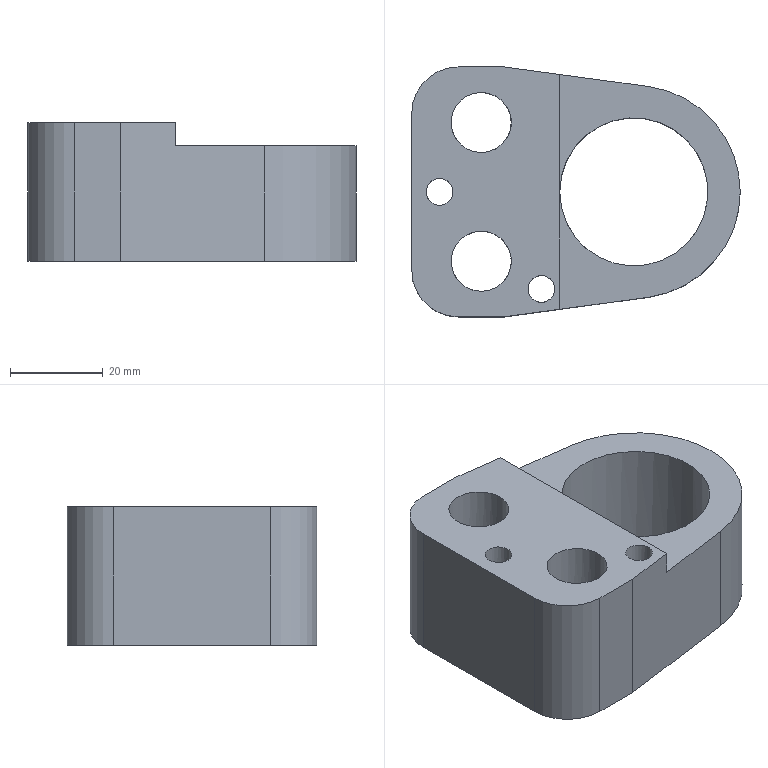Part | NX | features solid 2 | 1 solid | 25 faces | box 71.007 x 54.004 x 30 mm | volume 55355 mm3 | plane 13 | cylinder 12 | commonest cylinder face diameters 5.8 x2 8 x2 13 x2 19 x2 20 x2 32 x1
STEP:
#1=CARTESIAN_POINT('',(-440.164,-179.961,113.));
#2=VERTEX_POINT('',#1);
#3=CARTESIAN_POINT('',(-428.165,-178.332,113.));
#4=VERTEX_POINT('',#3);
#5=CARTESIAN_POINT('',(-420.346,-177.27,113.));
#6=DIRECTION('',(0.9909,0.1345,0.));
#7=VECTOR('',#6,1000.);
#8=LINE('',#5,#7);
#9=EDGE_CURVE('',#2,#4,#8,.T.);
#10=ORIENTED_EDGE('',*,*,#9,.T.);
#11=CARTESIAN_POINT('',(-428.185,-127.581,113.));
#12=VERTEX_POINT('',#11);
#13=CARTESIAN_POINT('',(-428.175,-152.956,113.));
#14=DIRECTION('',(-0.000407,1.,0.));
#15=VECTOR('',#14,1000.);
#16=LINE('',#13,#15);
#17=EDGE_CURVE('',#4,#12,#16,.T.);
#18=ORIENTED_EDGE('',*,*,#17,.T.);
#19=CARTESIAN_POINT('',(-440.186,-125.961,113.));
#20=VERTEX_POINT('',#19);
#21=CARTESIAN_POINT('',(-420.366,-128.636,113.));
#22=DIRECTION('',(-0.991,0.1337,0.));
#23=VECTOR('',#22,1000.);
#24=LINE('',#21,#23);
#25=EDGE_CURVE('',#12,#20,#24,.T.);
#26=ORIENTED_EDGE('',*,*,#25,.T.);
#27=CARTESIAN_POINT('',(-450.186,-125.965,113.));
#28=VERTEX_POINT('',#27);
#29=CARTESIAN_POINT('',(-424.641,-125.955,113.));
#30=DIRECTION('',(1.,0.000407,0.));
#31=VECTOR('',#30,1000.);
#32=LINE('',#29,#31);
#33=EDGE_CURVE('',#28,#20,#32,.T.);
#34=ORIENTED_EDGE('',*,*,#33,.F.);
#35=CARTESIAN_POINT('',(-460.182,-135.969,113.));
#36=VERTEX_POINT('',#35);
#37=CARTESIAN_POINT('',(-450.182,-135.965,113.));
#38=DIRECTION('',(0.,0.,1.));
#39=DIRECTION('',(1.,0.,0.));
#40=AXIS2_PLACEMENT_3D('',#37,#38,#39);
#41=CIRCLE('',#40,10.);
#42=EDGE_CURVE('',#28,#36,#41,.T.);
#43=ORIENTED_EDGE('',*,*,#42,.T.);
#44=CARTESIAN_POINT('',(-460.168,-169.969,113.));
#45=VERTEX_POINT('',#44);
#46=CARTESIAN_POINT('',(-460.175,-152.969,113.));
#47=DIRECTION('',(-0.000407,1.,0.));
#48=VECTOR('',#47,1000.);
#49=LINE('',#46,#48);
#50=EDGE_CURVE('',#45,#36,#49,.T.);
#51=ORIENTED_EDGE('',*,*,#50,.F.);
#52=CARTESIAN_POINT('',(-450.164,-179.965,113.));
#53=VERTEX_POINT('',#52);
#54=CARTESIAN_POINT('',(-450.168,-169.965,113.));
#55=DIRECTION('',(0.,0.,1.));
#56=DIRECTION('',(1.,0.,0.));
#57=AXIS2_PLACEMENT_3D('',#54,#55,#56);
#58=CIRCLE('',#57,10.);
#59=EDGE_CURVE('',#45,#53,#58,.T.);
#60=ORIENTED_EDGE('',*,*,#59,.T.);
#61=CARTESIAN_POINT('',(-424.619,-179.955,113.));
#62=DIRECTION('',(-1.,-0.000407,0.));
#63=VECTOR('',#62,1000.);
#64=LINE('',#61,#63);
#65=EDGE_CURVE('',#2,#53,#64,.T.);
#66=ORIENTED_EDGE('',*,*,#65,.F.);
#67=EDGE_LOOP('',(#10,#18,#26,#34,#43,#51,#60,#66));
#68=FACE_BOUND('',#67,.T.);
#69=CARTESIAN_POINT('',(-454.176,-150.067,113.));
#70=VERTEX_POINT('',#69);
#71=CARTESIAN_POINT('',(-454.175,-152.967,113.));
#72=DIRECTION('',(0.,0.,-1.));
#73=DIRECTION('',(-0.000407,1.,0.));
#74=AXIS2_PLACEMENT_3D('',#71,#72,#73);
#75=CIRCLE('',#74,2.9);
#76=EDGE_CURVE('',#70,#70,#75,.T.);
#77=ORIENTED_EDGE('',*,*,#76,.T.);
#78=EDGE_LOOP('',(#77));
#79=FACE_BOUND('',#78,.T.);
#80=CARTESIAN_POINT('',(-432.168,-171.058,113.));
#81=VERTEX_POINT('',#80);
#82=CARTESIAN_POINT('',(-432.167,-173.958,113.));
#83=DIRECTION('',(0.,0.,-1.));
#84=DIRECTION('',(-0.000407,1.,0.));
#85=AXIS2_PLACEMENT_3D('',#82,#83,#84);
#86=CIRCLE('',#85,2.9);
#87=EDGE_CURVE('',#81,#81,#86,.T.);
#88=ORIENTED_EDGE('',*,*,#87,.T.);
#89=EDGE_LOOP('',(#88));
#90=FACE_BOUND('',#89,.T.);
#91=CARTESIAN_POINT('',(-445.172,-161.463,113.));
#92=VERTEX_POINT('',#91);
#93=CARTESIAN_POINT('',(-445.169,-167.963,113.));
#94=DIRECTION('',(0.,0.,-1.));
#95=DIRECTION('',(-0.000407,1.,0.));
#96=AXIS2_PLACEMENT_3D('',#93,#94,#95);
#97=CIRCLE('',#96,6.5);
#98=EDGE_CURVE('',#92,#92,#97,.T.);
#99=ORIENTED_EDGE('',*,*,#98,.T.);
#100=EDGE_LOOP('',(#99));
#101=FACE_BOUND('',#100,.T.);
#102=CARTESIAN_POINT('',(-445.184,-131.463,113.));
#103=VERTEX_POINT('',#102);
#104=CARTESIAN_POINT('',(-445.181,-137.963,113.));
#105=DIRECTION('',(0.,0.,-1.));
#106=DIRECTION('',(-0.000407,1.,0.));
#107=AXIS2_PLACEMENT_3D('',#104,#105,#106);
#108=CIRCLE('',#107,6.5);
#109=EDGE_CURVE('',#103,#103,#108,.T.);
#110=ORIENTED_EDGE('',*,*,#109,.T.);
#111=EDGE_LOOP('',(#110));
#112=FACE_BOUND('',#111,.T.);
#113=CARTESIAN_POINT('',(-424.63,-152.955,113.));
#114=DIRECTION('',(0.,0.,1.));
#115=DIRECTION('',(0.000407,-1.,0.));
#116=AXIS2_PLACEMENT_3D('',#113,#114,#115);
#117=PLANE('',#116);
#118=ADVANCED_FACE('',(#68,#79,#90,#101,#112),#117,.T.);
#119=CARTESIAN_POINT('',(-440.186,-125.961,83.));
#120=VERTEX_POINT('',#119);
#121=CARTESIAN_POINT('',(-440.186,-125.961,83.));
#122=DIRECTION('',(0.,0.,1.));
#123=VECTOR('',#122,1000.);
#124=LINE('',#121,#123);
#125=EDGE_CURVE('',#120,#20,#124,.T.);
#126=ORIENTED_EDGE('',*,*,#125,.F.);
#127=CARTESIAN_POINT('',(-450.186,-125.965,83.));
#128=VERTEX_POINT('',#127);
#129=CARTESIAN_POINT('',(-424.641,-125.955,83.));
#130=DIRECTION('',(-1.,-0.000407,0.));
#131=VECTOR('',#130,1000.);
#132=LINE('',#129,#131);
#133=EDGE_CURVE('',#120,#128,#132,.T.);
#134=ORIENTED_EDGE('',*,*,#133,.T.);
#135=CARTESIAN_POINT('',(-450.186,-125.965,83.));
#136=DIRECTION('',(0.,0.,1.));
#137=VECTOR('',#136,1000.);
#138=LINE('',#135,#137);
#139=EDGE_CURVE('',#128,#28,#138,.T.);
#140=ORIENTED_EDGE('',*,*,#139,.T.);
#141=ORIENTED_EDGE('',*,*,#33,.T.);
#142=EDGE_LOOP('',(#126,#134,#140,#141));
#143=FACE_BOUND('',#142,.T.);
#144=CARTESIAN_POINT('',(-424.641,-125.955,83.));
#145=DIRECTION('',(-0.000407,1.,0.));
#146=DIRECTION('',(0.,0.,1.));
#147=AXIS2_PLACEMENT_3D('',#144,#145,#146);
#148=PLANE('',#147);
#149=ADVANCED_FACE('',(#143),#148,.T.);
#150=CARTESIAN_POINT('',(-409.076,-175.74,83.));
#151=VERTEX_POINT('',#150);
#152=CARTESIAN_POINT('',(-440.164,-179.961,83.));
#153=VERTEX_POINT('',#152);
#154=CARTESIAN_POINT('',(-420.346,-177.27,83.));
#155=DIRECTION('',(-0.9909,-0.1345,0.));
#156=VECTOR('',#155,1000.);
#157=LINE('',#154,#156);
#158=EDGE_CURVE('',#151,#153,#157,.T.);
#159=ORIENTED_EDGE('',*,*,#158,.T.);
#160=CARTESIAN_POINT('',(-450.164,-179.965,83.));
#161=VERTEX_POINT('',#160);
#162=CARTESIAN_POINT('',(-424.619,-179.955,83.));
#163=DIRECTION('',(1.,0.000407,0.));
#164=VECTOR('',#163,1000.);
#165=LINE('',#162,#164);
#166=EDGE_CURVE('',#161,#153,#165,.T.);
#167=ORIENTED_EDGE('',*,*,#166,.F.);
#168=CARTESIAN_POINT('',(-460.168,-169.969,83.));
#169=VERTEX_POINT('',#168);
#170=CARTESIAN_POINT('',(-450.168,-169.965,83.));
#171=DIRECTION('',(0.,0.,-1.));
#172=DIRECTION('',(-1.,0.,0.));
#173=AXIS2_PLACEMENT_3D('',#170,#171,#172);
#174=CIRCLE('',#173,10.);
#175=EDGE_CURVE('',#161,#169,#174,.T.);
#176=ORIENTED_EDGE('',*,*,#175,.T.);
#177=CARTESIAN_POINT('',(-460.182,-135.969,83.));
#178=VERTEX_POINT('',#177);
#179=CARTESIAN_POINT('',(-460.175,-152.969,83.));
#180=DIRECTION('',(0.000407,-1.,0.));
#181=VECTOR('',#180,1000.);
#182=LINE('',#179,#181);
#183=EDGE_CURVE('',#178,#169,#182,.T.);
#184=ORIENTED_EDGE('',*,*,#183,.F.);
#185=CARTESIAN_POINT('',(-450.182,-135.965,83.));
#186=DIRECTION('',(0.,0.,-1.));
#187=DIRECTION('',(-1.,0.,0.));
#188=AXIS2_PLACEMENT_3D('',#185,#186,#187);
#189=CIRCLE('',#188,10.);
#190=EDGE_CURVE('',#178,#128,#189,.T.);
#191=ORIENTED_EDGE('',*,*,#190,.T.);
#192=ORIENTED_EDGE('',*,*,#133,.F.);
#193=CARTESIAN_POINT('',(-409.094,-130.157,83.));
#194=VERTEX_POINT('',#193);
#195=CARTESIAN_POINT('',(-420.366,-128.636,83.));
#196=DIRECTION('',(0.991,-0.1337,0.));
#197=VECTOR('',#196,1000.);
#198=LINE('',#195,#197);
#199=EDGE_CURVE('',#120,#194,#198,.T.);
#200=ORIENTED_EDGE('',*,*,#199,.T.);
#201=CARTESIAN_POINT('',(-412.175,-152.95,83.));
#202=DIRECTION('',(0.,0.,1.));
#203=DIRECTION('',(0.000407,-1.,0.));
#204=AXIS2_PLACEMENT_3D('',#201,#202,#203);
#205=CIRCLE('',#204,23.);
#206=EDGE_CURVE('',#151,#194,#205,.T.);
#207=ORIENTED_EDGE('',*,*,#206,.F.);
#208=EDGE_LOOP('',(#159,#167,#176,#184,#191,#192,#200,#207));
#209=FACE_BOUND('',#208,.T.);
#210=CARTESIAN_POINT('',(-454.174,-156.967,83.));
#211=VERTEX_POINT('',#210);
#212=CARTESIAN_POINT('',(-454.175,-152.967,83.));
#213=DIRECTION('',(0.,0.,1.));
#214=DIRECTION('',(0.000407,-1.,0.));
#215=AXIS2_PLACEMENT_3D('',#212,#213,#214);
#216=CIRCLE('',#215,4.);
#217=EDGE_CURVE('',#211,#211,#216,.T.);
#218=ORIENTED_EDGE('',*,*,#217,.T.);
#219=EDGE_LOOP('',(#218));
#220=FACE_BOUND('',#219,.T.);
#221=CARTESIAN_POINT('',(-432.165,-177.958,83.));
#222=VERTEX_POINT('',#221);
#223=CARTESIAN_POINT('',(-432.167,-173.958,83.));
#224=DIRECTION('',(0.,0.,1.));
#225=DIRECTION('',(0.000407,-1.,0.));
#226=AXIS2_PLACEMENT_3D('',#223,#224,#225);
#227=CIRCLE('',#226,4.);
#228=EDGE_CURVE('',#222,#222,#227,.T.);
#229=ORIENTED_EDGE('',*,*,#228,.T.);
#230=EDGE_LOOP('',(#229));
#231=FACE_BOUND('',#230,.T.);
#232=CARTESIAN_POINT('',(-445.165,-177.463,83.));
#233=VERTEX_POINT('',#232);
#234=CARTESIAN_POINT('',(-445.169,-167.963,83.));
#235=DIRECTION('',(0.,0.,1.));
#236=DIRECTION('',(0.000407,-1.,0.));
#237=AXIS2_PLACEMENT_3D('',#234,#235,#236);
#238=CIRCLE('',#237,9.5);
#239=EDGE_CURVE('',#233,#233,#238,.T.);
#240=ORIENTED_EDGE('',*,*,#239,.T.);
#241=EDGE_LOOP('',(#240));
#242=FACE_BOUND('',#241,.T.);
#243=CARTESIAN_POINT('',(-445.177,-147.463,83.));
#244=VERTEX_POINT('',#243);
#245=CARTESIAN_POINT('',(-445.181,-137.963,83.));
#246=DIRECTION('',(0.,0.,1.));
#247=DIRECTION('',(0.000407,-1.,0.));
#248=AXIS2_PLACEMENT_3D('',#245,#246,#247);
#249=CIRCLE('',#248,9.5);
#250=EDGE_CURVE('',#244,#244,#249,.T.);
#251=ORIENTED_EDGE('',*,*,#250,.T.);
#252=EDGE_LOOP('',(#251));
#253=FACE_BOUND('',#252,.T.);
#254=CARTESIAN_POINT('',(-412.169,-168.95,83.));
#255=VERTEX_POINT('',#254);
#256=CARTESIAN_POINT('',(-412.175,-152.95,83.));
#257=DIRECTION('',(0.,0.,1.));
#258=DIRECTION('',(0.000407,-1.,0.));
#259=AXIS2_PLACEMENT_3D('',#256,#257,#258);
#260=CIRCLE('',#259,16.);
#261=EDGE_CURVE('',#255,#255,#260,.T.);
#262=ORIENTED_EDGE('',*,*,#261,.T.);
#263=EDGE_LOOP('',(#262));
#264=FACE_BOUND('',#263,.T.);
#265=CARTESIAN_POINT('',(-424.63,-152.955,83.));
#266=DIRECTION('',(0.,0.,-1.));
#267=DIRECTION('',(-0.000407,1.,0.));
#268=AXIS2_PLACEMENT_3D('',#265,#266,#267);
#269=PLANE('',#268);
#270=ADVANCED_FACE('',(#209,#220,#231,#242,#253,#264),#269,.T.);
#271=CARTESIAN_POINT('',(-440.164,-179.961,83.));
#272=DIRECTION('',(0.,0.,1.));
#273=VECTOR('',#272,1000.);
#274=LINE('',#271,#273);
#275=EDGE_CURVE('',#153,#2,#274,.T.);
#276=ORIENTED_EDGE('',*,*,#275,.T.);
#277=ORIENTED_EDGE('',*,*,#65,.T.);
#278=CARTESIAN_POINT('',(-450.164,-179.965,83.));
#279=DIRECTION('',(0.,0.,1.));
#280=VECTOR('',#279,1000.);
#281=LINE('',#278,#280);
#282=EDGE_CURVE('',#53,#161,#281,.F.);
#283=ORIENTED_EDGE('',*,*,#282,.T.);
#284=ORIENTED_EDGE('',*,*,#166,.T.);
#285=EDGE_LOOP('',(#276,#277,#283,#284));
#286=FACE_BOUND('',#285,.T.);
#287=CARTESIAN_POINT('',(-424.619,-179.955,83.));
#288=DIRECTION('',(0.000407,-1.,0.));
#289=DIRECTION('',(0.,0.,-1.));
#290=AXIS2_PLACEMENT_3D('',#287,#288,#289);
#291=PLANE('',#290);
#292=ADVANCED_FACE('',(#286),#291,.T.);
#293=CARTESIAN_POINT('',(-409.076,-175.74,108.));
#294=VERTEX_POINT('',#293);
#295=CARTESIAN_POINT('',(-409.094,-130.157,108.));
#296=VERTEX_POINT('',#295);
#297=CARTESIAN_POINT('',(-412.175,-152.95,108.));
#298=DIRECTION('',(0.,0.,-1.));
#299=DIRECTION('',(-1.,0.,0.));
#300=AXIS2_PLACEMENT_3D('',#297,#298,#299);
#301=CIRCLE('',#300,23.);
#302=EDGE_CURVE('',#294,#296,#301,.F.);
#303=ORIENTED_EDGE('',*,*,#302,.F.);
#304=CARTESIAN_POINT('',(-409.076,-175.74,113.));
#305=DIRECTION('',(0.,0.,-1.));
#306=VECTOR('',#305,1000.);
#307=LINE('',#304,#306);
#308=EDGE_CURVE('',#294,#151,#307,.T.);
#309=ORIENTED_EDGE('',*,*,#308,.T.);
#310=ORIENTED_EDGE('',*,*,#206,.T.);
#311=CARTESIAN_POINT('',(-409.094,-130.157,113.));
#312=DIRECTION('',(0.,0.,-1.));
#313=VECTOR('',#312,1000.);
#314=LINE('',#311,#313);
#315=EDGE_CURVE('',#194,#296,#314,.F.);
#316=ORIENTED_EDGE('',*,*,#315,.T.);
#317=EDGE_LOOP('',(#303,#309,#310,#316));
#318=FACE_BOUND('',#317,.T.);
#319=CARTESIAN_POINT('',(-412.175,-152.95,113.));
#320=DIRECTION('',(0.,0.,-1.));
#321=DIRECTION('',(-0.000407,1.,0.));
#322=AXIS2_PLACEMENT_3D('',#319,#320,#321);
#323=CYLINDRICAL_SURFACE('',#322,23.);
#324=ADVANCED_FACE('',(#318),#323,.T.);
#325=ORIENTED_EDGE('',*,*,#183,.T.);
#326=CARTESIAN_POINT('',(-460.168,-169.969,83.));
#327=DIRECTION('',(0.,0.,1.));
#328=VECTOR('',#327,1000.);
#329=LINE('',#326,#328);
#330=EDGE_CURVE('',#169,#45,#329,.T.);
#331=ORIENTED_EDGE('',*,*,#330,.T.);
#332=ORIENTED_EDGE('',*,*,#50,.T.);
#333=CARTESIAN_POINT('',(-460.182,-135.969,83.));
#334=DIRECTION('',(0.,0.,1.));
#335=VECTOR('',#334,1000.);
#336=LINE('',#333,#335);
#337=EDGE_CURVE('',#36,#178,#336,.F.);
#338=ORIENTED_EDGE('',*,*,#337,.T.);
#339=EDGE_LOOP('',(#325,#331,#332,#338));
#340=FACE_BOUND('',#339,.T.);
#341=CARTESIAN_POINT('',(-460.175,-152.969,83.));
#342=DIRECTION('',(-1.,-0.000407,0.));
#343=DIRECTION('',(0.,0.,-1.));
#344=AXIS2_PLACEMENT_3D('',#341,#342,#343);
#345=PLANE('',#344);
#346=ADVANCED_FACE('',(#340),#345,.T.);
#347=ORIENTED_EDGE('',*,*,#17,.F.);
#348=CARTESIAN_POINT('',(-428.165,-178.332,108.));
#349=VERTEX_POINT('',#348);
#350=CARTESIAN_POINT('',(-428.165,-178.332,108.));
#351=DIRECTION('',(0.,0.,-1.));
#352=VECTOR('',#351,1000.);
#353=LINE('',#350,#352);
#354=EDGE_CURVE('',#4,#349,#353,.T.);
#355=ORIENTED_EDGE('',*,*,#354,.T.);
#356=CARTESIAN_POINT('',(-428.175,-152.956,108.));
#357=VERTEX_POINT('',#356);
#358=CARTESIAN_POINT('',(-428.175,-152.956,108.));
#359=DIRECTION('',(0.000407,-1.,0.));
#360=VECTOR('',#359,1000.);
#361=LINE('',#358,#360);
#362=EDGE_CURVE('',#357,#349,#361,.T.);
#363=ORIENTED_EDGE('',*,*,#362,.F.);
#364=CARTESIAN_POINT('',(-428.185,-127.581,108.));
#365=VERTEX_POINT('',#364);
#366=CARTESIAN_POINT('',(-428.175,-152.956,108.));
#367=DIRECTION('',(0.000407,-1.,0.));
#368=VECTOR('',#367,1000.);
#369=LINE('',#366,#368);
#370=EDGE_CURVE('',#365,#357,#369,.T.);
#371=ORIENTED_EDGE('',*,*,#370,.F.);
#372=CARTESIAN_POINT('',(-428.185,-127.581,108.));
#373=DIRECTION('',(0.,0.,1.));
#374=VECTOR('',#373,1000.);
#375=LINE('',#372,#374);
#376=EDGE_CURVE('',#365,#12,#375,.T.);
#377=ORIENTED_EDGE('',*,*,#376,.T.);
#378=EDGE_LOOP('',(#347,#355,#363,#371,#377));
#379=FACE_BOUND('',#378,.T.);
#380=CARTESIAN_POINT('',(-428.175,-152.956,108.));
#381=DIRECTION('',(-1.,-0.000407,0.));
#382=DIRECTION('',(0.,0.,-1.));
#383=AXIS2_PLACEMENT_3D('',#380,#381,#382);
#384=PLANE('',#383);
#385=ADVANCED_FACE('',(#379),#384,.F.);
#386=ORIENTED_EDGE('',*,*,#362,.T.);
#387=CARTESIAN_POINT('',(-397.788,-174.207,108.));
#388=DIRECTION('',(0.9909,0.1345,0.));
#389=VECTOR('',#388,1000.);
#390=LINE('',#387,#389);
#391=EDGE_CURVE('',#349,#294,#390,.T.);
#392=ORIENTED_EDGE('',*,*,#391,.T.);
#393=ORIENTED_EDGE('',*,*,#302,.T.);
#394=CARTESIAN_POINT('',(-397.805,-131.68,108.));
#395=DIRECTION('',(-0.991,0.1337,0.));
#396=VECTOR('',#395,1000.);
#397=LINE('',#394,#396);
#398=EDGE_CURVE('',#296,#365,#397,.T.);
#399=ORIENTED_EDGE('',*,*,#398,.T.);
#400=ORIENTED_EDGE('',*,*,#370,.T.);
#401=CARTESIAN_POINT('',(-412.175,-152.95,108.));
#402=DIRECTION('',(0.,0.,-1.));
#403=DIRECTION('',(-0.000407,1.,0.));
#404=AXIS2_PLACEMENT_3D('',#401,#402,#403);
#405=CIRCLE('',#404,16.);
#406=EDGE_CURVE('',#357,#357,#405,.T.);
#407=ORIENTED_EDGE('',*,*,#406,.T.);
#408=EDGE_LOOP('',(#386,#392,#393,#399,#400,#407));
#409=FACE_BOUND('',#408,.T.);
#410=CARTESIAN_POINT('',(-400.675,-152.945,108.));
#411=DIRECTION('',(0.,0.,-1.));
#412=DIRECTION('',(-0.000407,1.,0.));
#413=AXIS2_PLACEMENT_3D('',#410,#411,#412);
#414=PLANE('',#413);
#415=ADVANCED_FACE('',(#409),#414,.F.);
#416=ORIENTED_EDGE('',*,*,#261,.F.);
#417=EDGE_LOOP('',(#416));
#418=FACE_BOUND('',#417,.T.);
#419=ORIENTED_EDGE('',*,*,#406,.F.);
#420=EDGE_LOOP('',(#419));
#421=FACE_BOUND('',#420,.T.);
#422=CARTESIAN_POINT('',(-412.175,-152.95,108.));
#423=DIRECTION('',(0.,0.,-1.));
#424=DIRECTION('',(-0.000407,1.,0.));
#425=AXIS2_PLACEMENT_3D('',#422,#423,#424);
#426=CYLINDRICAL_SURFACE('',#425,16.);
#427=ADVANCED_FACE('',(#418,#421),#426,.F.);
#428=CARTESIAN_POINT('',(-438.681,-137.963,97.));
#429=VERTEX_POINT('',#428);
#430=CARTESIAN_POINT('',(-445.181,-137.963,97.));
#431=DIRECTION('',(0.,0.,1.));
#432=DIRECTION('',(1.,0.,0.));
#433=AXIS2_PLACEMENT_3D('',#430,#431,#432);
#434=CIRCLE('',#433,6.5);
#435=EDGE_CURVE('',#429,#429,#434,.F.);
#436=ORIENTED_EDGE('',*,*,#435,.T.);
#437=EDGE_LOOP('',(#436));
#438=FACE_BOUND('',#437,.T.);
#439=ORIENTED_EDGE('',*,*,#109,.F.);
#440=EDGE_LOOP('',(#439));
#441=FACE_BOUND('',#440,.T.);
#442=CARTESIAN_POINT('',(-445.181,-137.963,113.));
#443=DIRECTION('',(0.,0.,-1.));
#444=DIRECTION('',(-0.000407,1.,0.));
#445=AXIS2_PLACEMENT_3D('',#442,#443,#444);
#446=CYLINDRICAL_SURFACE('',#445,6.5);
#447=ADVANCED_FACE('',(#438,#441),#446,.F.);
#448=CARTESIAN_POINT('',(-445.185,-128.463,97.));
#449=VERTEX_POINT('',#448);
#450=CARTESIAN_POINT('',(-445.181,-137.963,97.));
#451=DIRECTION('',(0.,0.,-1.));
#452=DIRECTION('',(-0.000407,1.,0.));
#453=AXIS2_PLACEMENT_3D('',#450,#451,#452);
#454=CIRCLE('',#453,9.5);
#455=EDGE_CURVE('',#449,#449,#454,.T.);
#456=ORIENTED_EDGE('',*,*,#455,.T.);
#457=EDGE_LOOP('',(#456));
#458=FACE_BOUND('',#457,.T.);
#459=ORIENTED_EDGE('',*,*,#435,.F.);
#460=EDGE_LOOP('',(#459));
#461=FACE_BOUND('',#460,.T.);
#462=CARTESIAN_POINT('',(-445.181,-137.963,97.));
#463=DIRECTION('',(0.,0.,1.));
#464=DIRECTION('',(0.000407,-1.,0.));
#465=AXIS2_PLACEMENT_3D('',#462,#463,#464);
#466=PLANE('',#465);
#467=ADVANCED_FACE('',(#458,#461),#466,.F.);
#468=ORIENTED_EDGE('',*,*,#250,.F.);
#469=EDGE_LOOP('',(#468));
#470=FACE_BOUND('',#469,.T.);
#471=ORIENTED_EDGE('',*,*,#455,.F.);
#472=EDGE_LOOP('',(#471));
#473=FACE_BOUND('',#472,.T.);
#474=CARTESIAN_POINT('',(-445.181,-137.963,97.));
#475=DIRECTION('',(0.,0.,-1.));
#476=DIRECTION('',(-0.000407,1.,0.));
#477=AXIS2_PLACEMENT_3D('',#474,#475,#476);
#478=CYLINDRICAL_SURFACE('',#477,9.5);
#479=ADVANCED_FACE('',(#470,#473),#478,.F.);
#480=CARTESIAN_POINT('',(-438.669,-167.963,97.));
#481=VERTEX_POINT('',#480);
#482=CARTESIAN_POINT('',(-445.169,-167.963,97.));
#483=DIRECTION('',(0.,0.,1.));
#484=DIRECTION('',(1.,0.,0.));
#485=AXIS2_PLACEMENT_3D('',#482,#483,#484);
#486=CIRCLE('',#485,6.5);
#487=EDGE_CURVE('',#481,#481,#486,.F.);
#488=ORIENTED_EDGE('',*,*,#487,.T.);
#489=EDGE_LOOP('',(#488));
#490=FACE_BOUND('',#489,.T.);
#491=ORIENTED_EDGE('',*,*,#98,.F.);
#492=EDGE_LOOP('',(#491));
#493=FACE_BOUND('',#492,.T.);
#494=CARTESIAN_POINT('',(-445.169,-167.963,113.));
#495=DIRECTION('',(0.,0.,-1.));
#496=DIRECTION('',(-0.000407,1.,0.));
#497=AXIS2_PLACEMENT_3D('',#494,#495,#496);
#498=CYLINDRICAL_SURFACE('',#497,6.5);
#499=ADVANCED_FACE('',(#490,#493),#498,.F.);
#500=CARTESIAN_POINT('',(-445.173,-158.463,97.));
#501=VERTEX_POINT('',#500);
#502=CARTESIAN_POINT('',(-445.169,-167.963,97.));
#503=DIRECTION('',(0.,0.,-1.));
#504=DIRECTION('',(-0.000407,1.,0.));
#505=AXIS2_PLACEMENT_3D('',#502,#503,#504);
#506=CIRCLE('',#505,9.5);
#507=EDGE_CURVE('',#501,#501,#506,.T.);
#508=ORIENTED_EDGE('',*,*,#507,.T.);
#509=EDGE_LOOP('',(#508));
#510=FACE_BOUND('',#509,.T.);
#511=ORIENTED_EDGE('',*,*,#487,.F.);
#512=EDGE_LOOP('',(#511));
#513=FACE_BOUND('',#512,.T.);
#514=CARTESIAN_POINT('',(-445.169,-167.963,97.));
#515=DIRECTION('',(0.,0.,1.));
#516=DIRECTION('',(0.000407,-1.,0.));
#517=AXIS2_PLACEMENT_3D('',#514,#515,#516);
#518=PLANE('',#517);
#519=ADVANCED_FACE('',(#510,#513),#518,.F.);
#520=ORIENTED_EDGE('',*,*,#239,.F.);
#521=EDGE_LOOP('',(#520));
#522=FACE_BOUND('',#521,.T.);
#523=ORIENTED_EDGE('',*,*,#507,.F.);
#524=EDGE_LOOP('',(#523));
#525=FACE_BOUND('',#524,.T.);
#526=CARTESIAN_POINT('',(-445.169,-167.963,97.));
#527=DIRECTION('',(0.,0.,-1.));
#528=DIRECTION('',(-0.000407,1.,0.));
#529=AXIS2_PLACEMENT_3D('',#526,#527,#528);
#530=CYLINDRICAL_SURFACE('',#529,9.5);
#531=ADVANCED_FACE('',(#522,#525),#530,.F.);
#532=CARTESIAN_POINT('',(-429.267,-173.958,103.));
#533=VERTEX_POINT('',#532);
#534=CARTESIAN_POINT('',(-432.167,-173.958,103.));
#535=DIRECTION('',(0.,0.,1.));
#536=DIRECTION('',(1.,0.,0.));
#537=AXIS2_PLACEMENT_3D('',#534,#535,#536);
#538=CIRCLE('',#537,2.9);
#539=EDGE_CURVE('',#533,#533,#538,.F.);
#540=ORIENTED_EDGE('',*,*,#539,.T.);
#541=EDGE_LOOP('',(#540));
#542=FACE_BOUND('',#541,.T.);
#543=ORIENTED_EDGE('',*,*,#87,.F.);
#544=EDGE_LOOP('',(#543));
#545=FACE_BOUND('',#544,.T.);
#546=CARTESIAN_POINT('',(-432.167,-173.958,113.));
#547=DIRECTION('',(0.,0.,-1.));
#548=DIRECTION('',(-0.000407,1.,0.));
#549=AXIS2_PLACEMENT_3D('',#546,#547,#548);
#550=CYLINDRICAL_SURFACE('',#549,2.9);
#551=ADVANCED_FACE('',(#542,#545),#550,.F.);
#552=CARTESIAN_POINT('',(-432.168,-169.958,103.));
#553=VERTEX_POINT('',#552);
#554=CARTESIAN_POINT('',(-432.167,-173.958,103.));
#555=DIRECTION('',(0.,0.,-1.));
#556=DIRECTION('',(-0.000407,1.,0.));
#557=AXIS2_PLACEMENT_3D('',#554,#555,#556);
#558=CIRCLE('',#557,4.);
#559=EDGE_CURVE('',#553,#553,#558,.T.);
#560=ORIENTED_EDGE('',*,*,#559,.T.);
#561=EDGE_LOOP('',(#560));
#562=FACE_BOUND('',#561,.T.);
#563=ORIENTED_EDGE('',*,*,#539,.F.);
#564=EDGE_LOOP('',(#563));
#565=FACE_BOUND('',#564,.T.);
#566=CARTESIAN_POINT('',(-432.167,-173.958,103.));
#567=DIRECTION('',(0.,0.,1.));
#568=DIRECTION('',(0.000407,-1.,0.));
#569=AXIS2_PLACEMENT_3D('',#566,#567,#568);
#570=PLANE('',#569);
#571=ADVANCED_FACE('',(#562,#565),#570,.F.);
#572=ORIENTED_EDGE('',*,*,#228,.F.);
#573=EDGE_LOOP('',(#572));
#574=FACE_BOUND('',#573,.T.);
#575=ORIENTED_EDGE('',*,*,#559,.F.);
#576=EDGE_LOOP('',(#575));
#577=FACE_BOUND('',#576,.T.);
#578=CARTESIAN_POINT('',(-432.167,-173.958,103.));
#579=DIRECTION('',(0.,0.,-1.));
#580=DIRECTION('',(-0.000407,1.,0.));
#581=AXIS2_PLACEMENT_3D('',#578,#579,#580);
#582=CYLINDRICAL_SURFACE('',#581,4.);
#583=ADVANCED_FACE('',(#574,#577),#582,.F.);
#584=CARTESIAN_POINT('',(-451.275,-152.967,103.));
#585=VERTEX_POINT('',#584);
#586=CARTESIAN_POINT('',(-454.175,-152.967,103.));
#587=DIRECTION('',(0.,0.,1.));
#588=DIRECTION('',(1.,0.,0.));
#589=AXIS2_PLACEMENT_3D('',#586,#587,#588);
#590=CIRCLE('',#589,2.9);
#591=EDGE_CURVE('',#585,#585,#590,.F.);
#592=ORIENTED_EDGE('',*,*,#591,.T.);
#593=EDGE_LOOP('',(#592));
#594=FACE_BOUND('',#593,.T.);
#595=ORIENTED_EDGE('',*,*,#76,.F.);
#596=EDGE_LOOP('',(#595));
#597=FACE_BOUND('',#596,.T.);
#598=CARTESIAN_POINT('',(-454.175,-152.967,113.));
#599=DIRECTION('',(0.,0.,-1.));
#600=DIRECTION('',(-0.000407,1.,0.));
#601=AXIS2_PLACEMENT_3D('',#598,#599,#600);
#602=CYLINDRICAL_SURFACE('',#601,2.9);
#603=ADVANCED_FACE('',(#594,#597),#602,.F.);
#604=CARTESIAN_POINT('',(-454.177,-148.967,103.));
#605=VERTEX_POINT('',#604);
#606=CARTESIAN_POINT('',(-454.175,-152.967,103.));
#607=DIRECTION('',(0.,0.,-1.));
#608=DIRECTION('',(-0.000407,1.,0.));
#609=AXIS2_PLACEMENT_3D('',#606,#607,#608);
#610=CIRCLE('',#609,4.);
#611=EDGE_CURVE('',#605,#605,#610,.T.);
#612=ORIENTED_EDGE('',*,*,#611,.T.);
#613=EDGE_LOOP('',(#612));
#614=FACE_BOUND('',#613,.T.);
#615=ORIENTED_EDGE('',*,*,#591,.F.);
#616=EDGE_LOOP('',(#615));
#617=FACE_BOUND('',#616,.T.);
#618=CARTESIAN_POINT('',(-454.175,-152.967,103.));
#619=DIRECTION('',(0.,0.,1.));
#620=DIRECTION('',(0.000407,-1.,0.));
#621=AXIS2_PLACEMENT_3D('',#618,#619,#620);
#622=PLANE('',#621);
#623=ADVANCED_FACE('',(#614,#617),#622,.F.);
#624=ORIENTED_EDGE('',*,*,#217,.F.);
#625=EDGE_LOOP('',(#624));
#626=FACE_BOUND('',#625,.T.);
#627=ORIENTED_EDGE('',*,*,#611,.F.);
#628=EDGE_LOOP('',(#627));
#629=FACE_BOUND('',#628,.T.);
#630=CARTESIAN_POINT('',(-454.175,-152.967,103.));
#631=DIRECTION('',(0.,0.,-1.));
#632=DIRECTION('',(-0.000407,1.,0.));
#633=AXIS2_PLACEMENT_3D('',#630,#631,#632);
#634=CYLINDRICAL_SURFACE('',#633,4.);
#635=ADVANCED_FACE('',(#626,#629),#634,.F.);
#636=ORIENTED_EDGE('',*,*,#175,.F.);
#637=ORIENTED_EDGE('',*,*,#282,.F.);
#638=ORIENTED_EDGE('',*,*,#59,.F.);
#639=ORIENTED_EDGE('',*,*,#330,.F.);
#640=EDGE_LOOP('',(#636,#637,#638,#639));
#641=FACE_BOUND('',#640,.T.);
#642=CARTESIAN_POINT('',(-450.168,-169.965,83.));
#643=DIRECTION('',(0.,0.,1.));
#644=DIRECTION('',(1.,0.,0.));
#645=AXIS2_PLACEMENT_3D('',#642,#643,#644);
#646=CYLINDRICAL_SURFACE('',#645,10.);
#647=ADVANCED_FACE('',(#641),#646,.T.);
#648=ORIENTED_EDGE('',*,*,#190,.F.);
#649=ORIENTED_EDGE('',*,*,#337,.F.);
#650=ORIENTED_EDGE('',*,*,#42,.F.);
#651=ORIENTED_EDGE('',*,*,#139,.F.);
#652=EDGE_LOOP('',(#648,#649,#650,#651));
#653=FACE_BOUND('',#652,.T.);
#654=CARTESIAN_POINT('',(-450.182,-135.965,83.));
#655=DIRECTION('',(0.,0.,1.));
#656=DIRECTION('',(1.,0.,0.));
#657=AXIS2_PLACEMENT_3D('',#654,#655,#656);
#658=CYLINDRICAL_SURFACE('',#657,10.);
#659=ADVANCED_FACE('',(#653),#658,.T.);
#660=ORIENTED_EDGE('',*,*,#315,.F.);
#661=ORIENTED_EDGE('',*,*,#199,.F.);
#662=ORIENTED_EDGE('',*,*,#125,.T.);
#663=ORIENTED_EDGE('',*,*,#25,.F.);
#664=ORIENTED_EDGE('',*,*,#376,.F.);
#665=ORIENTED_EDGE('',*,*,#398,.F.);
#666=EDGE_LOOP('',(#660,#661,#662,#663,#664,#665));
#667=FACE_BOUND('',#666,.T.);
#668=CARTESIAN_POINT('',(-420.366,-128.636,83.));
#669=DIRECTION('',(-0.1337,-0.991,0.));
#670=DIRECTION('',(0.,0.,-1.));
#671=AXIS2_PLACEMENT_3D('',#668,#669,#670);
#672=PLANE('',#671);
#673=ADVANCED_FACE('',(#667),#672,.F.);
#674=ORIENTED_EDGE('',*,*,#308,.F.);
#675=ORIENTED_EDGE('',*,*,#391,.F.);
#676=ORIENTED_EDGE('',*,*,#354,.F.);
#677=ORIENTED_EDGE('',*,*,#9,.F.);
#678=ORIENTED_EDGE('',*,*,#275,.F.);
#679=ORIENTED_EDGE('',*,*,#158,.F.);
#680=EDGE_LOOP('',(#674,#675,#676,#677,#678,#679));
#681=FACE_BOUND('',#680,.T.);
#682=CARTESIAN_POINT('',(-420.346,-177.27,83.));
#683=DIRECTION('',(-0.1345,0.9909,0.));
#684=DIRECTION('',(0.,0.,1.));
#685=AXIS2_PLACEMENT_3D('',#682,#683,#684);
#686=PLANE('',#685);
#687=ADVANCED_FACE('',(#681),#686,.F.);
#688=CLOSED_SHELL('',(#118,#149,#270,#292,#324,#346,#385,#415,#427,#447,#467,#479,#499,#519,#531,#551,#571,#583,#603,#623,#635,#647,#659,#673,#687));
#689=MANIFOLD_SOLID_BREP('',#688);
#690=(LENGTH_UNIT()NAMED_UNIT(*)SI_UNIT(.MILLI.,.METRE.));
#691=UNCERTAINTY_MEASURE_WITH_UNIT(LENGTH_MEASURE(0.00001),#690,'','');
#692=(NAMED_UNIT(*)PLANE_ANGLE_UNIT()SI_UNIT($,.RADIAN.));
#693=(NAMED_UNIT(*)SI_UNIT($,.STERADIAN.)SOLID_ANGLE_UNIT());
#694=(GEOMETRIC_REPRESENTATION_CONTEXT(3)GLOBAL_UNCERTAINTY_ASSIGNED_CONTEXT((#691))GLOBAL_UNIT_ASSIGNED_CONTEXT((#690,#692,#693))REPRESENTATION_CONTEXT('',''));
#695=ADVANCED_BREP_SHAPE_REPRESENTATION('',(#689),#694);